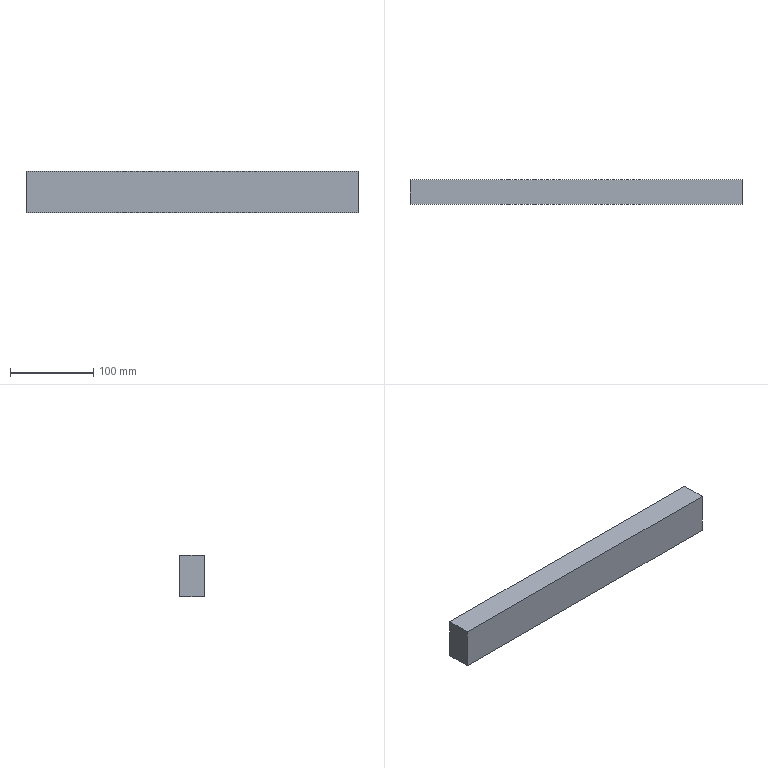Part | NX | features solid 2 | 1 solid | 6 faces | box 400 x 30 x 50 mm | volume 600000 mm3 | plane 6
STEP:
#1=CARTESIAN_POINT('',(570.,225.,225.));
#2=VERTEX_POINT('',#1);
#3=CARTESIAN_POINT('',(570.,195.,225.));
#4=VERTEX_POINT('',#3);
#5=CARTESIAN_POINT('',(570.,210.,225.));
#6=DIRECTION('',(0.,1.,0.));
#7=VECTOR('',#6,1000.);
#8=LINE('',#5,#7);
#9=EDGE_CURVE('',#2,#4,#8,.F.);
#10=ORIENTED_EDGE('',*,*,#9,.F.);
#11=CARTESIAN_POINT('',(970.,225.,225.));
#12=VERTEX_POINT('',#11);
#13=CARTESIAN_POINT('',(500.,225.,225.));
#14=DIRECTION('',(1.,0.,0.));
#15=VECTOR('',#14,1000.);
#16=LINE('',#13,#15);
#17=EDGE_CURVE('',#2,#12,#16,.T.);
#18=ORIENTED_EDGE('',*,*,#17,.T.);
#19=CARTESIAN_POINT('',(970.,195.,225.));
#20=VERTEX_POINT('',#19);
#21=CARTESIAN_POINT('',(970.,195.,225.));
#22=DIRECTION('',(0.,-1.,0.));
#23=VECTOR('',#22,1000.);
#24=LINE('',#21,#23);
#25=EDGE_CURVE('',#12,#20,#24,.T.);
#26=ORIENTED_EDGE('',*,*,#25,.T.);
#27=CARTESIAN_POINT('',(500.,195.,225.));
#28=DIRECTION('',(-1.,0.,0.));
#29=VECTOR('',#28,1000.);
#30=LINE('',#27,#29);
#31=EDGE_CURVE('',#20,#4,#30,.T.);
#32=ORIENTED_EDGE('',*,*,#31,.T.);
#33=EDGE_LOOP('',(#10,#18,#26,#32));
#34=FACE_BOUND('',#33,.T.);
#35=CARTESIAN_POINT('',(-620.,-610.,225.));
#36=DIRECTION('',(0.,0.,-1.));
#37=DIRECTION('',(-1.,0.,0.));
#38=AXIS2_PLACEMENT_3D('',#35,#36,#37);
#39=PLANE('',#38);
#40=ADVANCED_FACE('',(#34),#39,.T.);
#41=CARTESIAN_POINT('',(570.,195.,275.));
#42=VERTEX_POINT('',#41);
#43=CARTESIAN_POINT('',(970.,195.,275.));
#44=VERTEX_POINT('',#43);
#45=CARTESIAN_POINT('',(-540.,195.,275.));
#46=DIRECTION('',(1.,0.,0.));
#47=VECTOR('',#46,1000.);
#48=LINE('',#45,#47);
#49=EDGE_CURVE('',#42,#44,#48,.T.);
#50=ORIENTED_EDGE('',*,*,#49,.T.);
#51=CARTESIAN_POINT('',(970.,225.,275.));
#52=VERTEX_POINT('',#51);
#53=CARTESIAN_POINT('',(970.,195.,275.));
#54=DIRECTION('',(0.,-1.,0.));
#55=VECTOR('',#54,1000.);
#56=LINE('',#53,#55);
#57=EDGE_CURVE('',#52,#44,#56,.T.);
#58=ORIENTED_EDGE('',*,*,#57,.F.);
#59=CARTESIAN_POINT('',(570.,225.,275.));
#60=VERTEX_POINT('',#59);
#61=CARTESIAN_POINT('',(-540.,225.,275.));
#62=DIRECTION('',(1.,0.,0.));
#63=VECTOR('',#62,1000.);
#64=LINE('',#61,#63);
#65=EDGE_CURVE('',#60,#52,#64,.T.);
#66=ORIENTED_EDGE('',*,*,#65,.F.);
#67=CARTESIAN_POINT('',(570.,210.,275.));
#68=DIRECTION('',(0.,1.,0.));
#69=VECTOR('',#68,1000.);
#70=LINE('',#67,#69);
#71=EDGE_CURVE('',#60,#42,#70,.F.);
#72=ORIENTED_EDGE('',*,*,#71,.T.);
#73=EDGE_LOOP('',(#50,#58,#66,#72));
#74=FACE_BOUND('',#73,.T.);
#75=CARTESIAN_POINT('',(-540.,-625.,275.));
#76=DIRECTION('',(0.,0.,-1.));
#77=DIRECTION('',(-1.,0.,0.));
#78=AXIS2_PLACEMENT_3D('',#75,#76,#77);
#79=PLANE('',#78);
#80=ADVANCED_FACE('',(#74),#79,.F.);
#81=ORIENTED_EDGE('',*,*,#25,.F.);
#82=CARTESIAN_POINT('',(970.,225.,155.));
#83=DIRECTION('',(0.,0.,-1.));
#84=VECTOR('',#83,1000.);
#85=LINE('',#82,#84);
#86=EDGE_CURVE('',#52,#12,#85,.T.);
#87=ORIENTED_EDGE('',*,*,#86,.F.);
#88=ORIENTED_EDGE('',*,*,#57,.T.);
#89=CARTESIAN_POINT('',(970.,195.,155.));
#90=DIRECTION('',(0.,0.,-1.));
#91=VECTOR('',#90,1000.);
#92=LINE('',#89,#91);
#93=EDGE_CURVE('',#44,#20,#92,.T.);
#94=ORIENTED_EDGE('',*,*,#93,.T.);
#95=EDGE_LOOP('',(#81,#87,#88,#94));
#96=FACE_BOUND('',#95,.T.);
#97=CARTESIAN_POINT('',(970.,195.,365.));
#98=DIRECTION('',(-1.,0.,0.));
#99=DIRECTION('',(0.,1.,0.));
#100=AXIS2_PLACEMENT_3D('',#97,#98,#99);
#101=PLANE('',#100);
#102=ADVANCED_FACE('',(#96),#101,.F.);
#103=ORIENTED_EDGE('',*,*,#86,.T.);
#104=ORIENTED_EDGE('',*,*,#17,.F.);
#105=CARTESIAN_POINT('',(570.,225.,155.));
#106=DIRECTION('',(0.,0.,-1.));
#107=VECTOR('',#106,1000.);
#108=LINE('',#105,#107);
#109=EDGE_CURVE('',#2,#60,#108,.F.);
#110=ORIENTED_EDGE('',*,*,#109,.T.);
#111=ORIENTED_EDGE('',*,*,#65,.T.);
#112=EDGE_LOOP('',(#103,#104,#110,#111));
#113=FACE_BOUND('',#112,.T.);
#114=CARTESIAN_POINT('',(500.,225.,155.));
#115=DIRECTION('',(0.,1.,0.));
#116=DIRECTION('',(0.,0.,-1.));
#117=AXIS2_PLACEMENT_3D('',#114,#115,#116);
#118=PLANE('',#117);
#119=ADVANCED_FACE('',(#113),#118,.T.);
#120=ORIENTED_EDGE('',*,*,#31,.F.);
#121=ORIENTED_EDGE('',*,*,#93,.F.);
#122=ORIENTED_EDGE('',*,*,#49,.F.);
#123=CARTESIAN_POINT('',(570.,195.,155.));
#124=DIRECTION('',(0.,0.,-1.));
#125=VECTOR('',#124,1000.);
#126=LINE('',#123,#125);
#127=EDGE_CURVE('',#4,#42,#126,.F.);
#128=ORIENTED_EDGE('',*,*,#127,.F.);
#129=EDGE_LOOP('',(#120,#121,#122,#128));
#130=FACE_BOUND('',#129,.T.);
#131=CARTESIAN_POINT('',(500.,195.,155.));
#132=DIRECTION('',(0.,1.,0.));
#133=DIRECTION('',(0.,0.,-1.));
#134=AXIS2_PLACEMENT_3D('',#131,#132,#133);
#135=PLANE('',#134);
#136=ADVANCED_FACE('',(#130),#135,.F.);
#137=ORIENTED_EDGE('',*,*,#109,.F.);
#138=ORIENTED_EDGE('',*,*,#9,.T.);
#139=ORIENTED_EDGE('',*,*,#127,.T.);
#140=ORIENTED_EDGE('',*,*,#71,.F.);
#141=EDGE_LOOP('',(#137,#138,#139,#140));
#142=FACE_BOUND('',#141,.T.);
#143=CARTESIAN_POINT('',(570.,210.,130.));
#144=DIRECTION('',(1.,0.,0.));
#145=DIRECTION('',(0.,0.,1.));
#146=AXIS2_PLACEMENT_3D('',#143,#144,#145);
#147=PLANE('',#146);
#148=ADVANCED_FACE('',(#142),#147,.F.);
#149=CLOSED_SHELL('',(#40,#80,#102,#119,#136,#148));
#150=MANIFOLD_SOLID_BREP('',#149);
#151=(LENGTH_UNIT()NAMED_UNIT(*)SI_UNIT(.MILLI.,.METRE.));
#152=UNCERTAINTY_MEASURE_WITH_UNIT(LENGTH_MEASURE(0.00001),#151,'','');
#153=(NAMED_UNIT(*)PLANE_ANGLE_UNIT()SI_UNIT($,.RADIAN.));
#154=(NAMED_UNIT(*)SI_UNIT($,.STERADIAN.)SOLID_ANGLE_UNIT());
#155=(GEOMETRIC_REPRESENTATION_CONTEXT(3)GLOBAL_UNCERTAINTY_ASSIGNED_CONTEXT((#152))GLOBAL_UNIT_ASSIGNED_CONTEXT((#151,#153,#154))REPRESENTATION_CONTEXT('',''));
#156=ADVANCED_BREP_SHAPE_REPRESENTATION('',(#150),#155);